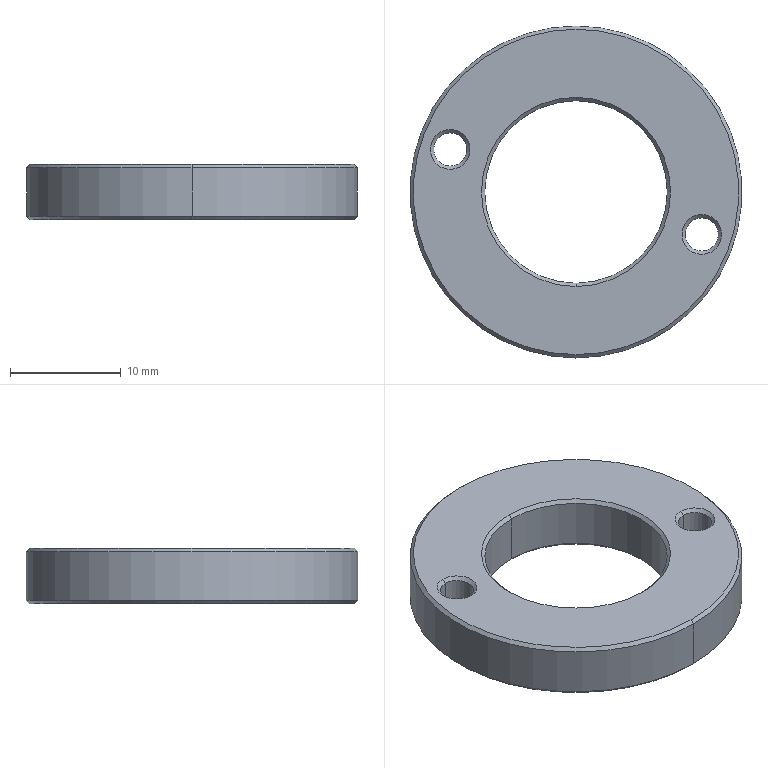Part | SolidWorks | features BaseBody 1 | 1 solid | 22 faces | box 30 x 30 x 5 mm | volume 2380 mm3 | cone 12 | cylinder 8 | plane 2 | commonest cylinder face diameters 3 x4 16.5 x2 30 x2
STEP:
#1=CARTESIAN_POINT('',(700.535,23.972,-71.23));
#2=VERTEX_POINT('',#1);
#3=CARTESIAN_POINT('',(700.535,53.372,-71.23));
#4=VERTEX_POINT('',#3);
#5=CARTESIAN_POINT('',(700.535,38.672,-71.23));
#6=DIRECTION('',(0.000000001,-0.000000003,1.));
#7=DIRECTION('',(0.,-1.,-0.000000003));
#8=AXIS2_PLACEMENT_3D('',#5,#6,#7);
#9=CIRCLE('',#8,14.7);
#10=EDGE_CURVE('',#2,#4,#9,.T.);
#11=ORIENTED_EDGE('',*,*,#10,.T.);
#12=CARTESIAN_POINT('',(700.535,53.672,-70.93));
#13=VERTEX_POINT('',#12);
#14=CARTESIAN_POINT('',(700.535,53.672,-70.93));
#15=DIRECTION('',(0.000000001,0.7071,0.7071));
#16=VECTOR('',#15,1000.);
#17=LINE('',#14,#16);
#18=EDGE_CURVE('',#4,#13,#17,.T.);
#19=ORIENTED_EDGE('',*,*,#18,.T.);
#20=CARTESIAN_POINT('',(700.535,23.672,-70.93));
#21=VERTEX_POINT('',#20);
#22=CARTESIAN_POINT('',(700.535,38.672,-70.93));
#23=DIRECTION('',(-0.000000001,0.000000003,-1.));
#24=DIRECTION('',(0.004352,-1.,-0.000000003));
#25=AXIS2_PLACEMENT_3D('',#22,#23,#24);
#26=CIRCLE('',#25,15.);
#27=EDGE_CURVE('',#13,#21,#26,.T.);
#28=ORIENTED_EDGE('',*,*,#27,.T.);
#29=CARTESIAN_POINT('',(700.535,23.672,-70.93));
#30=DIRECTION('',(0.000000001,-0.7071,0.7071));
#31=VECTOR('',#30,1000.);
#32=LINE('',#29,#31);
#33=EDGE_CURVE('',#2,#21,#32,.T.);
#34=ORIENTED_EDGE('',*,*,#33,.F.);
#35=EDGE_LOOP('',(#11,#19,#28,#34));
#36=FACE_OUTER_BOUND('',#35,.T.);
#37=CARTESIAN_POINT('',(700.535,38.672,-70.93));
#38=DIRECTION('',(0.000000001,-0.000000003,1.));
#39=DIRECTION('',(0.,-1.,-0.000000003));
#40=AXIS2_PLACEMENT_3D('',#37,#38,#39);
#41=CONICAL_SURFACE('',#40,15.,0.7854);
#42=ADVANCED_FACE('',(#36),#41,.T.);
#43=CARTESIAN_POINT('',(711.903,33.329,-71.23));
#44=VERTEX_POINT('',#43);
#45=CARTESIAN_POINT('',(711.903,36.329,-71.23));
#46=VERTEX_POINT('',#45);
#47=CARTESIAN_POINT('',(711.903,34.829,-71.23));
#48=DIRECTION('',(-0.000000001,0.000000003,-1.));
#49=DIRECTION('',(0.,-1.,-0.000000003));
#50=AXIS2_PLACEMENT_3D('',#47,#48,#49);
#51=CIRCLE('',#50,1.5);
#52=EDGE_CURVE('',#44,#46,#51,.T.);
#53=ORIENTED_EDGE('',*,*,#52,.T.);
#54=CARTESIAN_POINT('',(711.903,36.329,-66.53));
#55=VERTEX_POINT('',#54);
#56=CARTESIAN_POINT('',(711.903,36.329,-66.23));
#57=DIRECTION('',(0.000000001,-0.000000003,1.));
#58=VECTOR('',#57,1000.);
#59=LINE('',#56,#58);
#60=EDGE_CURVE('',#46,#55,#59,.T.);
#61=ORIENTED_EDGE('',*,*,#60,.T.);
#62=CARTESIAN_POINT('',(711.903,33.329,-66.53));
#63=VERTEX_POINT('',#62);
#64=CARTESIAN_POINT('',(711.903,34.829,-66.53));
#65=DIRECTION('',(-0.000000001,0.000000003,-1.));
#66=DIRECTION('',(0.,-1.,-0.000000003));
#67=AXIS2_PLACEMENT_3D('',#64,#65,#66);
#68=CIRCLE('',#67,1.5);
#69=EDGE_CURVE('',#63,#55,#68,.T.);
#70=ORIENTED_EDGE('',*,*,#69,.F.);
#71=CARTESIAN_POINT('',(711.903,33.329,-66.23));
#72=DIRECTION('',(0.000000001,-0.000000003,1.));
#73=VECTOR('',#72,1000.);
#74=LINE('',#71,#73);
#75=EDGE_CURVE('',#44,#63,#74,.T.);
#76=ORIENTED_EDGE('',*,*,#75,.F.);
#77=EDGE_LOOP('',(#53,#61,#70,#76));
#78=FACE_OUTER_BOUND('',#77,.T.);
#79=CARTESIAN_POINT('',(711.903,34.829,-66.23));
#80=DIRECTION('',(0.000000001,-0.000000003,1.));
#81=DIRECTION('',(0.,-1.,-0.000000003));
#82=AXIS2_PLACEMENT_3D('',#79,#80,#81);
#83=CYLINDRICAL_SURFACE('',#82,1.5);
#84=ADVANCED_FACE('',(#78),#83,.F.);
#85=CARTESIAN_POINT('',(689.167,41.015,-71.23));
#86=VERTEX_POINT('',#85);
#87=CARTESIAN_POINT('',(689.167,44.015,-71.23));
#88=VERTEX_POINT('',#87);
#89=CARTESIAN_POINT('',(689.167,42.515,-71.23));
#90=DIRECTION('',(-0.000000001,0.000000003,-1.));
#91=DIRECTION('',(0.,-1.,-0.000000003));
#92=AXIS2_PLACEMENT_3D('',#89,#90,#91);
#93=CIRCLE('',#92,1.5);
#94=EDGE_CURVE('',#86,#88,#93,.T.);
#95=ORIENTED_EDGE('',*,*,#94,.T.);
#96=CARTESIAN_POINT('',(689.167,44.015,-66.53));
#97=VERTEX_POINT('',#96);
#98=CARTESIAN_POINT('',(689.167,44.015,-66.23));
#99=DIRECTION('',(0.000000001,-0.000000003,1.));
#100=VECTOR('',#99,1000.);
#101=LINE('',#98,#100);
#102=EDGE_CURVE('',#88,#97,#101,.T.);
#103=ORIENTED_EDGE('',*,*,#102,.T.);
#104=CARTESIAN_POINT('',(689.167,41.015,-66.53));
#105=VERTEX_POINT('',#104);
#106=CARTESIAN_POINT('',(689.167,42.515,-66.53));
#107=DIRECTION('',(-0.000000001,0.000000003,-1.));
#108=DIRECTION('',(0.,-1.,-0.000000003));
#109=AXIS2_PLACEMENT_3D('',#106,#107,#108);
#110=CIRCLE('',#109,1.5);
#111=EDGE_CURVE('',#105,#97,#110,.T.);
#112=ORIENTED_EDGE('',*,*,#111,.F.);
#113=CARTESIAN_POINT('',(689.167,41.015,-66.23));
#114=DIRECTION('',(0.000000001,-0.000000003,1.));
#115=VECTOR('',#114,1000.);
#116=LINE('',#113,#115);
#117=EDGE_CURVE('',#86,#105,#116,.T.);
#118=ORIENTED_EDGE('',*,*,#117,.F.);
#119=EDGE_LOOP('',(#95,#103,#112,#118));
#120=FACE_OUTER_BOUND('',#119,.T.);
#121=CARTESIAN_POINT('',(689.167,42.515,-66.23));
#122=DIRECTION('',(0.000000001,-0.000000003,1.));
#123=DIRECTION('',(0.,-1.,-0.000000003));
#124=AXIS2_PLACEMENT_3D('',#121,#122,#123);
#125=CYLINDRICAL_SURFACE('',#124,1.5);
#126=ADVANCED_FACE('',(#120),#125,.F.);
#127=CARTESIAN_POINT('',(700.535,30.422,-70.93));
#128=VERTEX_POINT('',#127);
#129=CARTESIAN_POINT('',(700.535,46.922,-70.93));
#130=VERTEX_POINT('',#129);
#131=CARTESIAN_POINT('',(700.535,38.672,-70.93));
#132=DIRECTION('',(-0.000000001,0.000000003,-1.));
#133=DIRECTION('',(-0.004352,1.,0.000000003));
#134=AXIS2_PLACEMENT_3D('',#131,#132,#133);
#135=CIRCLE('',#134,8.25);
#136=EDGE_CURVE('',#128,#130,#135,.T.);
#137=ORIENTED_EDGE('',*,*,#136,.F.);
#138=CARTESIAN_POINT('',(700.535,30.122,-71.23));
#139=VERTEX_POINT('',#138);
#140=CARTESIAN_POINT('',(700.535,30.122,-71.23));
#141=DIRECTION('',(-0.000000001,-0.7071,-0.7071));
#142=VECTOR('',#141,1000.);
#143=LINE('',#140,#142);
#144=EDGE_CURVE('',#128,#139,#143,.T.);
#145=ORIENTED_EDGE('',*,*,#144,.T.);
#146=CARTESIAN_POINT('',(700.535,47.222,-71.23));
#147=VERTEX_POINT('',#146);
#148=CARTESIAN_POINT('',(700.535,38.672,-71.23));
#149=DIRECTION('',(-0.000000001,0.000000003,-1.));
#150=DIRECTION('',(0.,1.,0.000000003));
#151=AXIS2_PLACEMENT_3D('',#148,#149,#150);
#152=CIRCLE('',#151,8.55);
#153=EDGE_CURVE('',#139,#147,#152,.T.);
#154=ORIENTED_EDGE('',*,*,#153,.T.);
#155=CARTESIAN_POINT('',(700.535,47.222,-71.23));
#156=DIRECTION('',(-0.000000001,0.7071,-0.7071));
#157=VECTOR('',#156,1000.);
#158=LINE('',#155,#157);
#159=EDGE_CURVE('',#130,#147,#158,.T.);
#160=ORIENTED_EDGE('',*,*,#159,.F.);
#161=EDGE_LOOP('',(#137,#145,#154,#160));
#162=FACE_OUTER_BOUND('',#161,.T.);
#163=CARTESIAN_POINT('',(700.535,38.672,-71.23));
#164=DIRECTION('',(-0.000000001,0.000000003,-1.));
#165=DIRECTION('',(0.,1.,0.000000003));
#166=AXIS2_PLACEMENT_3D('',#163,#164,#165);
#167=CONICAL_SURFACE('',#166,8.55,0.7854);
#168=ADVANCED_FACE('',(#162),#167,.F.);
#169=CARTESIAN_POINT('',(700.535,53.672,-66.53));
#170=VERTEX_POINT('',#169);
#171=CARTESIAN_POINT('',(700.535,23.672,-66.53));
#172=VERTEX_POINT('',#171);
#173=CARTESIAN_POINT('',(700.535,38.672,-66.53));
#174=DIRECTION('',(-0.000000001,0.000000003,-1.));
#175=DIRECTION('',(0.,1.,0.000000003));
#176=AXIS2_PLACEMENT_3D('',#173,#174,#175);
#177=CIRCLE('',#176,15.);
#178=EDGE_CURVE('',#170,#172,#177,.T.);
#179=ORIENTED_EDGE('',*,*,#178,.T.);
#180=CARTESIAN_POINT('',(700.535,23.672,-71.23));
#181=DIRECTION('',(-0.000000001,0.000000003,-1.));
#182=VECTOR('',#181,1000.);
#183=LINE('',#180,#182);
#184=EDGE_CURVE('',#172,#21,#183,.T.);
#185=ORIENTED_EDGE('',*,*,#184,.T.);
#186=ORIENTED_EDGE('',*,*,#27,.F.);
#187=CARTESIAN_POINT('',(700.535,53.672,-71.23));
#188=DIRECTION('',(-0.000000001,0.000000003,-1.));
#189=VECTOR('',#188,1000.);
#190=LINE('',#187,#189);
#191=EDGE_CURVE('',#170,#13,#190,.T.);
#192=ORIENTED_EDGE('',*,*,#191,.F.);
#193=EDGE_LOOP('',(#179,#185,#186,#192));
#194=FACE_OUTER_BOUND('',#193,.T.);
#195=CARTESIAN_POINT('',(700.535,38.672,-71.23));
#196=DIRECTION('',(-0.000000001,0.000000003,-1.));
#197=DIRECTION('',(0.,1.,0.000000003));
#198=AXIS2_PLACEMENT_3D('',#195,#196,#197);
#199=CYLINDRICAL_SURFACE('',#198,15.);
#200=ADVANCED_FACE('',(#194),#199,.T.);
#201=ORIENTED_EDGE('',*,*,#69,.T.);
#202=CARTESIAN_POINT('',(711.903,36.629,-66.23));
#203=VERTEX_POINT('',#202);
#204=CARTESIAN_POINT('',(711.903,36.629,-66.23));
#205=DIRECTION('',(0.000000001,0.7071,0.7071));
#206=VECTOR('',#205,1000.);
#207=LINE('',#204,#206);
#208=EDGE_CURVE('',#55,#203,#207,.T.);
#209=ORIENTED_EDGE('',*,*,#208,.T.);
#210=CARTESIAN_POINT('',(711.903,33.029,-66.23));
#211=VERTEX_POINT('',#210);
#212=CARTESIAN_POINT('',(711.903,34.829,-66.23));
#213=DIRECTION('',(-0.000000001,0.000000003,-1.));
#214=DIRECTION('',(0.,-1.,-0.000000003));
#215=AXIS2_PLACEMENT_3D('',#212,#213,#214);
#216=CIRCLE('',#215,1.8);
#217=EDGE_CURVE('',#211,#203,#216,.T.);
#218=ORIENTED_EDGE('',*,*,#217,.F.);
#219=CARTESIAN_POINT('',(711.903,33.029,-66.23));
#220=DIRECTION('',(0.000000001,-0.7071,0.7071));
#221=VECTOR('',#220,1000.);
#222=LINE('',#219,#221);
#223=EDGE_CURVE('',#63,#211,#222,.T.);
#224=ORIENTED_EDGE('',*,*,#223,.F.);
#225=EDGE_LOOP('',(#201,#209,#218,#224));
#226=FACE_OUTER_BOUND('',#225,.T.);
#227=CARTESIAN_POINT('',(711.903,34.829,-66.23));
#228=DIRECTION('',(0.000000001,-0.000000003,1.));
#229=DIRECTION('',(0.,-1.,-0.000000003));
#230=AXIS2_PLACEMENT_3D('',#227,#228,#229);
#231=CONICAL_SURFACE('',#230,1.8,0.7854);
#232=ADVANCED_FACE('',(#226),#231,.F.);
#233=ORIENTED_EDGE('',*,*,#111,.T.);
#234=CARTESIAN_POINT('',(689.167,44.315,-66.23));
#235=VERTEX_POINT('',#234);
#236=CARTESIAN_POINT('',(689.167,44.315,-66.23));
#237=DIRECTION('',(0.000000001,0.7071,0.7071));
#238=VECTOR('',#237,1000.);
#239=LINE('',#236,#238);
#240=EDGE_CURVE('',#97,#235,#239,.T.);
#241=ORIENTED_EDGE('',*,*,#240,.T.);
#242=CARTESIAN_POINT('',(689.167,40.715,-66.23));
#243=VERTEX_POINT('',#242);
#244=CARTESIAN_POINT('',(689.167,42.515,-66.23));
#245=DIRECTION('',(-0.000000001,0.000000003,-1.));
#246=DIRECTION('',(0.,-1.,-0.000000003));
#247=AXIS2_PLACEMENT_3D('',#244,#245,#246);
#248=CIRCLE('',#247,1.8);
#249=EDGE_CURVE('',#243,#235,#248,.T.);
#250=ORIENTED_EDGE('',*,*,#249,.F.);
#251=CARTESIAN_POINT('',(689.167,40.715,-66.23));
#252=DIRECTION('',(0.000000001,-0.7071,0.7071));
#253=VECTOR('',#252,1000.);
#254=LINE('',#251,#253);
#255=EDGE_CURVE('',#105,#243,#254,.T.);
#256=ORIENTED_EDGE('',*,*,#255,.F.);
#257=EDGE_LOOP('',(#233,#241,#250,#256));
#258=FACE_OUTER_BOUND('',#257,.T.);
#259=CARTESIAN_POINT('',(689.167,42.515,-66.23));
#260=DIRECTION('',(0.000000001,-0.000000003,1.));
#261=DIRECTION('',(0.,-1.,-0.000000003));
#262=AXIS2_PLACEMENT_3D('',#259,#260,#261);
#263=CONICAL_SURFACE('',#262,1.8,0.7854);
#264=ADVANCED_FACE('',(#258),#263,.F.);
#265=CARTESIAN_POINT('',(700.535,30.422,-66.53));
#266=VERTEX_POINT('',#265);
#267=CARTESIAN_POINT('',(700.535,46.922,-66.53));
#268=VERTEX_POINT('',#267);
#269=CARTESIAN_POINT('',(700.535,38.672,-66.53));
#270=DIRECTION('',(-0.000000001,0.000000003,-1.));
#271=DIRECTION('',(0.,1.,0.000000003));
#272=AXIS2_PLACEMENT_3D('',#269,#270,#271);
#273=CIRCLE('',#272,8.25);
#274=EDGE_CURVE('',#266,#268,#273,.T.);
#275=ORIENTED_EDGE('',*,*,#274,.F.);
#276=CARTESIAN_POINT('',(700.535,30.422,-68.73));
#277=DIRECTION('',(-0.000000001,0.000000003,-1.));
#278=VECTOR('',#277,1000.);
#279=LINE('',#276,#278);
#280=EDGE_CURVE('',#266,#128,#279,.T.);
#281=ORIENTED_EDGE('',*,*,#280,.T.);
#282=ORIENTED_EDGE('',*,*,#136,.T.);
#283=CARTESIAN_POINT('',(700.535,46.922,-68.73));
#284=DIRECTION('',(-0.000000001,0.000000003,-1.));
#285=VECTOR('',#284,1000.);
#286=LINE('',#283,#285);
#287=EDGE_CURVE('',#268,#130,#286,.T.);
#288=ORIENTED_EDGE('',*,*,#287,.F.);
#289=EDGE_LOOP('',(#275,#281,#282,#288));
#290=FACE_OUTER_BOUND('',#289,.T.);
#291=CARTESIAN_POINT('',(700.535,38.672,-68.73));
#292=DIRECTION('',(-0.000000001,0.000000003,-1.));
#293=DIRECTION('',(0.,1.,0.000000003));
#294=AXIS2_PLACEMENT_3D('',#291,#292,#293);
#295=CYLINDRICAL_SURFACE('',#294,8.25);
#296=ADVANCED_FACE('',(#290),#295,.F.);
#297=CARTESIAN_POINT('',(700.535,53.372,-66.23));
#298=VERTEX_POINT('',#297);
#299=CARTESIAN_POINT('',(700.535,23.972,-66.23));
#300=VERTEX_POINT('',#299);
#301=CARTESIAN_POINT('',(700.535,38.672,-66.23));
#302=DIRECTION('',(-0.000000001,0.000000003,-1.));
#303=DIRECTION('',(0.,1.,0.000000003));
#304=AXIS2_PLACEMENT_3D('',#301,#302,#303);
#305=CIRCLE('',#304,14.7);
#306=EDGE_CURVE('',#298,#300,#305,.T.);
#307=ORIENTED_EDGE('',*,*,#306,.T.);
#308=CARTESIAN_POINT('',(700.535,23.672,-66.53));
#309=DIRECTION('',(-0.000000001,-0.7071,-0.7071));
#310=VECTOR('',#309,1000.);
#311=LINE('',#308,#310);
#312=EDGE_CURVE('',#300,#172,#311,.T.);
#313=ORIENTED_EDGE('',*,*,#312,.T.);
#314=ORIENTED_EDGE('',*,*,#178,.F.);
#315=CARTESIAN_POINT('',(700.535,53.672,-66.53));
#316=DIRECTION('',(-0.000000001,0.7071,-0.7071));
#317=VECTOR('',#316,1000.);
#318=LINE('',#315,#317);
#319=EDGE_CURVE('',#298,#170,#318,.T.);
#320=ORIENTED_EDGE('',*,*,#319,.F.);
#321=EDGE_LOOP('',(#307,#313,#314,#320));
#322=FACE_OUTER_BOUND('',#321,.T.);
#323=CARTESIAN_POINT('',(700.535,38.672,-66.53));
#324=DIRECTION('',(-0.000000001,0.000000003,-1.));
#325=DIRECTION('',(0.,1.,0.000000003));
#326=AXIS2_PLACEMENT_3D('',#323,#324,#325);
#327=CONICAL_SURFACE('',#326,15.,0.7854);
#328=ADVANCED_FACE('',(#322),#327,.T.);
#329=ORIENTED_EDGE('',*,*,#274,.T.);
#330=CARTESIAN_POINT('',(700.535,47.222,-66.23));
#331=VERTEX_POINT('',#330);
#332=CARTESIAN_POINT('',(700.535,47.222,-66.23));
#333=DIRECTION('',(0.000000001,0.7071,0.7071));
#334=VECTOR('',#333,1000.);
#335=LINE('',#332,#334);
#336=EDGE_CURVE('',#268,#331,#335,.T.);
#337=ORIENTED_EDGE('',*,*,#336,.T.);
#338=CARTESIAN_POINT('',(700.535,30.122,-66.23));
#339=VERTEX_POINT('',#338);
#340=CARTESIAN_POINT('',(700.535,38.672,-66.23));
#341=DIRECTION('',(-0.000000001,0.000000003,-1.));
#342=DIRECTION('',(0.,-1.,-0.000000003));
#343=AXIS2_PLACEMENT_3D('',#340,#341,#342);
#344=CIRCLE('',#343,8.55);
#345=EDGE_CURVE('',#339,#331,#344,.T.);
#346=ORIENTED_EDGE('',*,*,#345,.F.);
#347=CARTESIAN_POINT('',(700.535,30.122,-66.23));
#348=DIRECTION('',(0.000000001,-0.7071,0.7071));
#349=VECTOR('',#348,1000.);
#350=LINE('',#347,#349);
#351=EDGE_CURVE('',#266,#339,#350,.T.);
#352=ORIENTED_EDGE('',*,*,#351,.F.);
#353=EDGE_LOOP('',(#329,#337,#346,#352));
#354=FACE_OUTER_BOUND('',#353,.T.);
#355=CARTESIAN_POINT('',(700.535,38.672,-66.23));
#356=DIRECTION('',(0.000000001,-0.000000003,1.));
#357=DIRECTION('',(0.,-1.,-0.000000003));
#358=AXIS2_PLACEMENT_3D('',#355,#356,#357);
#359=CONICAL_SURFACE('',#358,8.55,0.7854);
#360=ADVANCED_FACE('',(#354),#359,.F.);
#361=ORIENTED_EDGE('',*,*,#10,.F.);
#362=CARTESIAN_POINT('',(700.535,38.672,-71.23));
#363=DIRECTION('',(0.000000001,-0.000000003,1.));
#364=DIRECTION('',(0.,-1.,-0.000000003));
#365=AXIS2_PLACEMENT_3D('',#362,#363,#364);
#366=CIRCLE('',#365,14.7);
#367=EDGE_CURVE('',#4,#2,#366,.T.);
#368=ORIENTED_EDGE('',*,*,#367,.F.);
#369=EDGE_LOOP('',(#361,#368));
#370=FACE_OUTER_BOUND('',#369,.T.);
#371=ORIENTED_EDGE('',*,*,#52,.F.);
#372=CARTESIAN_POINT('',(711.903,34.829,-71.23));
#373=DIRECTION('',(-0.000000001,0.000000003,-1.));
#374=DIRECTION('',(0.,-1.,-0.000000003));
#375=AXIS2_PLACEMENT_3D('',#372,#373,#374);
#376=CIRCLE('',#375,1.5);
#377=EDGE_CURVE('',#46,#44,#376,.T.);
#378=ORIENTED_EDGE('',*,*,#377,.F.);
#379=EDGE_LOOP('',(#371,#378));
#380=FACE_BOUND('',#379,.T.);
#381=ORIENTED_EDGE('',*,*,#94,.F.);
#382=CARTESIAN_POINT('',(689.167,42.515,-71.23));
#383=DIRECTION('',(-0.000000001,0.000000003,-1.));
#384=DIRECTION('',(0.,-1.,-0.000000003));
#385=AXIS2_PLACEMENT_3D('',#382,#383,#384);
#386=CIRCLE('',#385,1.5);
#387=EDGE_CURVE('',#88,#86,#386,.T.);
#388=ORIENTED_EDGE('',*,*,#387,.F.);
#389=EDGE_LOOP('',(#381,#388));
#390=FACE_BOUND('',#389,.T.);
#391=CARTESIAN_POINT('',(700.535,38.672,-71.23));
#392=DIRECTION('',(-0.000000001,0.000000003,-1.));
#393=DIRECTION('',(0.,1.,0.000000003));
#394=AXIS2_PLACEMENT_3D('',#391,#392,#393);
#395=CIRCLE('',#394,8.55);
#396=EDGE_CURVE('',#147,#139,#395,.T.);
#397=ORIENTED_EDGE('',*,*,#396,.F.);
#398=ORIENTED_EDGE('',*,*,#153,.F.);
#399=EDGE_LOOP('',(#397,#398));
#400=FACE_BOUND('',#399,.T.);
#401=CARTESIAN_POINT('',(700.535,38.672,-71.23));
#402=DIRECTION('',(0.000000001,-0.000000003,1.));
#403=DIRECTION('',(0.,-1.,-0.000000003));
#404=AXIS2_PLACEMENT_3D('',#401,#402,#403);
#405=PLANE('',#404);
#406=ADVANCED_FACE('',(#370,#380,#390,#400),#405,.F.);
#407=ORIENTED_EDGE('',*,*,#18,.F.);
#408=ORIENTED_EDGE('',*,*,#367,.T.);
#409=ORIENTED_EDGE('',*,*,#33,.T.);
#410=CARTESIAN_POINT('',(700.535,38.672,-70.93));
#411=DIRECTION('',(-0.000000001,0.000000003,-1.));
#412=DIRECTION('',(0.004352,-1.,-0.000000003));
#413=AXIS2_PLACEMENT_3D('',#410,#411,#412);
#414=CIRCLE('',#413,15.);
#415=EDGE_CURVE('',#21,#13,#414,.T.);
#416=ORIENTED_EDGE('',*,*,#415,.T.);
#417=EDGE_LOOP('',(#407,#408,#409,#416));
#418=FACE_OUTER_BOUND('',#417,.T.);
#419=CARTESIAN_POINT('',(700.535,38.672,-70.93));
#420=DIRECTION('',(0.000000001,-0.000000003,1.));
#421=DIRECTION('',(0.,-1.,-0.000000003));
#422=AXIS2_PLACEMENT_3D('',#419,#420,#421);
#423=CONICAL_SURFACE('',#422,15.,0.7854);
#424=ADVANCED_FACE('',(#418),#423,.T.);
#425=ORIENTED_EDGE('',*,*,#60,.F.);
#426=ORIENTED_EDGE('',*,*,#377,.T.);
#427=ORIENTED_EDGE('',*,*,#75,.T.);
#428=CARTESIAN_POINT('',(711.903,34.829,-66.53));
#429=DIRECTION('',(-0.000000001,0.000000003,-1.));
#430=DIRECTION('',(0.,-1.,-0.000000003));
#431=AXIS2_PLACEMENT_3D('',#428,#429,#430);
#432=CIRCLE('',#431,1.5);
#433=EDGE_CURVE('',#55,#63,#432,.T.);
#434=ORIENTED_EDGE('',*,*,#433,.F.);
#435=EDGE_LOOP('',(#425,#426,#427,#434));
#436=FACE_OUTER_BOUND('',#435,.T.);
#437=CARTESIAN_POINT('',(711.903,34.829,-66.23));
#438=DIRECTION('',(0.000000001,-0.000000003,1.));
#439=DIRECTION('',(0.,-1.,-0.000000003));
#440=AXIS2_PLACEMENT_3D('',#437,#438,#439);
#441=CYLINDRICAL_SURFACE('',#440,1.5);
#442=ADVANCED_FACE('',(#436),#441,.F.);
#443=ORIENTED_EDGE('',*,*,#102,.F.);
#444=ORIENTED_EDGE('',*,*,#387,.T.);
#445=ORIENTED_EDGE('',*,*,#117,.T.);
#446=CARTESIAN_POINT('',(689.167,42.515,-66.53));
#447=DIRECTION('',(-0.000000001,0.000000003,-1.));
#448=DIRECTION('',(0.,-1.,-0.000000003));
#449=AXIS2_PLACEMENT_3D('',#446,#447,#448);
#450=CIRCLE('',#449,1.5);
#451=EDGE_CURVE('',#97,#105,#450,.T.);
#452=ORIENTED_EDGE('',*,*,#451,.F.);
#453=EDGE_LOOP('',(#443,#444,#445,#452));
#454=FACE_OUTER_BOUND('',#453,.T.);
#455=CARTESIAN_POINT('',(689.167,42.515,-66.23));
#456=DIRECTION('',(0.000000001,-0.000000003,1.));
#457=DIRECTION('',(0.,-1.,-0.000000003));
#458=AXIS2_PLACEMENT_3D('',#455,#456,#457);
#459=CYLINDRICAL_SURFACE('',#458,1.5);
#460=ADVANCED_FACE('',(#454),#459,.F.);
#461=ORIENTED_EDGE('',*,*,#144,.F.);
#462=CARTESIAN_POINT('',(700.535,38.672,-70.93));
#463=DIRECTION('',(-0.000000001,0.000000003,-1.));
#464=DIRECTION('',(-0.004352,1.,0.000000003));
#465=AXIS2_PLACEMENT_3D('',#462,#463,#464);
#466=CIRCLE('',#465,8.25);
#467=EDGE_CURVE('',#130,#128,#466,.T.);
#468=ORIENTED_EDGE('',*,*,#467,.F.);
#469=ORIENTED_EDGE('',*,*,#159,.T.);
#470=ORIENTED_EDGE('',*,*,#396,.T.);
#471=EDGE_LOOP('',(#461,#468,#469,#470));
#472=FACE_OUTER_BOUND('',#471,.T.);
#473=CARTESIAN_POINT('',(700.535,38.672,-71.23));
#474=DIRECTION('',(-0.000000001,0.000000003,-1.));
#475=DIRECTION('',(0.,1.,0.000000003));
#476=AXIS2_PLACEMENT_3D('',#473,#474,#475);
#477=CONICAL_SURFACE('',#476,8.55,0.7854);
#478=ADVANCED_FACE('',(#472),#477,.F.);
#479=ORIENTED_EDGE('',*,*,#184,.F.);
#480=CARTESIAN_POINT('',(700.535,38.672,-66.53));
#481=DIRECTION('',(-0.000000001,0.000000003,-1.));
#482=DIRECTION('',(0.,1.,0.000000003));
#483=AXIS2_PLACEMENT_3D('',#480,#481,#482);
#484=CIRCLE('',#483,15.);
#485=EDGE_CURVE('',#172,#170,#484,.T.);
#486=ORIENTED_EDGE('',*,*,#485,.T.);
#487=ORIENTED_EDGE('',*,*,#191,.T.);
#488=ORIENTED_EDGE('',*,*,#415,.F.);
#489=EDGE_LOOP('',(#479,#486,#487,#488));
#490=FACE_OUTER_BOUND('',#489,.T.);
#491=CARTESIAN_POINT('',(700.535,38.672,-71.23));
#492=DIRECTION('',(-0.000000001,0.000000003,-1.));
#493=DIRECTION('',(0.,1.,0.000000003));
#494=AXIS2_PLACEMENT_3D('',#491,#492,#493);
#495=CYLINDRICAL_SURFACE('',#494,15.);
#496=ADVANCED_FACE('',(#490),#495,.T.);
#497=ORIENTED_EDGE('',*,*,#208,.F.);
#498=ORIENTED_EDGE('',*,*,#433,.T.);
#499=ORIENTED_EDGE('',*,*,#223,.T.);
#500=CARTESIAN_POINT('',(711.903,34.829,-66.23));
#501=DIRECTION('',(-0.000000001,0.000000003,-1.));
#502=DIRECTION('',(0.,-1.,-0.000000003));
#503=AXIS2_PLACEMENT_3D('',#500,#501,#502);
#504=CIRCLE('',#503,1.8);
#505=EDGE_CURVE('',#203,#211,#504,.T.);
#506=ORIENTED_EDGE('',*,*,#505,.F.);
#507=EDGE_LOOP('',(#497,#498,#499,#506));
#508=FACE_OUTER_BOUND('',#507,.T.);
#509=CARTESIAN_POINT('',(711.903,34.829,-66.23));
#510=DIRECTION('',(0.000000001,-0.000000003,1.));
#511=DIRECTION('',(0.,-1.,-0.000000003));
#512=AXIS2_PLACEMENT_3D('',#509,#510,#511);
#513=CONICAL_SURFACE('',#512,1.8,0.7854);
#514=ADVANCED_FACE('',(#508),#513,.F.);
#515=ORIENTED_EDGE('',*,*,#240,.F.);
#516=ORIENTED_EDGE('',*,*,#451,.T.);
#517=ORIENTED_EDGE('',*,*,#255,.T.);
#518=CARTESIAN_POINT('',(689.167,42.515,-66.23));
#519=DIRECTION('',(-0.000000001,0.000000003,-1.));
#520=DIRECTION('',(0.,-1.,-0.000000003));
#521=AXIS2_PLACEMENT_3D('',#518,#519,#520);
#522=CIRCLE('',#521,1.8);
#523=EDGE_CURVE('',#235,#243,#522,.T.);
#524=ORIENTED_EDGE('',*,*,#523,.F.);
#525=EDGE_LOOP('',(#515,#516,#517,#524));
#526=FACE_OUTER_BOUND('',#525,.T.);
#527=CARTESIAN_POINT('',(689.167,42.515,-66.23));
#528=DIRECTION('',(0.000000001,-0.000000003,1.));
#529=DIRECTION('',(0.,-1.,-0.000000003));
#530=AXIS2_PLACEMENT_3D('',#527,#528,#529);
#531=CONICAL_SURFACE('',#530,1.8,0.7854);
#532=ADVANCED_FACE('',(#526),#531,.F.);
#533=ORIENTED_EDGE('',*,*,#280,.F.);
#534=CARTESIAN_POINT('',(700.535,38.672,-66.53));
#535=DIRECTION('',(-0.000000001,0.000000003,-1.));
#536=DIRECTION('',(0.,1.,0.000000003));
#537=AXIS2_PLACEMENT_3D('',#534,#535,#536);
#538=CIRCLE('',#537,8.25);
#539=EDGE_CURVE('',#268,#266,#538,.T.);
#540=ORIENTED_EDGE('',*,*,#539,.F.);
#541=ORIENTED_EDGE('',*,*,#287,.T.);
#542=ORIENTED_EDGE('',*,*,#467,.T.);
#543=EDGE_LOOP('',(#533,#540,#541,#542));
#544=FACE_OUTER_BOUND('',#543,.T.);
#545=CARTESIAN_POINT('',(700.535,38.672,-68.73));
#546=DIRECTION('',(-0.000000001,0.000000003,-1.));
#547=DIRECTION('',(0.,1.,0.000000003));
#548=AXIS2_PLACEMENT_3D('',#545,#546,#547);
#549=CYLINDRICAL_SURFACE('',#548,8.25);
#550=ADVANCED_FACE('',(#544),#549,.F.);
#551=ORIENTED_EDGE('',*,*,#312,.F.);
#552=CARTESIAN_POINT('',(700.535,38.672,-66.23));
#553=DIRECTION('',(-0.000000001,0.000000003,-1.));
#554=DIRECTION('',(0.,1.,0.000000003));
#555=AXIS2_PLACEMENT_3D('',#552,#553,#554);
#556=CIRCLE('',#555,14.7);
#557=EDGE_CURVE('',#300,#298,#556,.T.);
#558=ORIENTED_EDGE('',*,*,#557,.T.);
#559=ORIENTED_EDGE('',*,*,#319,.T.);
#560=ORIENTED_EDGE('',*,*,#485,.F.);
#561=EDGE_LOOP('',(#551,#558,#559,#560));
#562=FACE_OUTER_BOUND('',#561,.T.);
#563=CARTESIAN_POINT('',(700.535,38.672,-66.53));
#564=DIRECTION('',(-0.000000001,0.000000003,-1.));
#565=DIRECTION('',(0.,1.,0.000000003));
#566=AXIS2_PLACEMENT_3D('',#563,#564,#565);
#567=CONICAL_SURFACE('',#566,15.,0.7854);
#568=ADVANCED_FACE('',(#562),#567,.T.);
#569=ORIENTED_EDGE('',*,*,#217,.T.);
#570=ORIENTED_EDGE('',*,*,#505,.T.);
#571=EDGE_LOOP('',(#569,#570));
#572=FACE_BOUND('',#571,.T.);
#573=ORIENTED_EDGE('',*,*,#345,.T.);
#574=CARTESIAN_POINT('',(700.535,38.672,-66.23));
#575=DIRECTION('',(-0.000000001,0.000000003,-1.));
#576=DIRECTION('',(0.,-1.,-0.000000003));
#577=AXIS2_PLACEMENT_3D('',#574,#575,#576);
#578=CIRCLE('',#577,8.55);
#579=EDGE_CURVE('',#331,#339,#578,.T.);
#580=ORIENTED_EDGE('',*,*,#579,.T.);
#581=EDGE_LOOP('',(#573,#580));
#582=FACE_BOUND('',#581,.T.);
#583=ORIENTED_EDGE('',*,*,#306,.F.);
#584=ORIENTED_EDGE('',*,*,#557,.F.);
#585=EDGE_LOOP('',(#583,#584));
#586=FACE_OUTER_BOUND('',#585,.T.);
#587=ORIENTED_EDGE('',*,*,#249,.T.);
#588=ORIENTED_EDGE('',*,*,#523,.T.);
#589=EDGE_LOOP('',(#587,#588));
#590=FACE_BOUND('',#589,.T.);
#591=CARTESIAN_POINT('',(700.535,38.672,-66.23));
#592=DIRECTION('',(0.000000001,-0.000000003,1.));
#593=DIRECTION('',(0.,-1.,-0.000000003));
#594=AXIS2_PLACEMENT_3D('',#591,#592,#593);
#595=PLANE('',#594);
#596=ADVANCED_FACE('',(#572,#582,#586,#590),#595,.T.);
#597=ORIENTED_EDGE('',*,*,#336,.F.);
#598=ORIENTED_EDGE('',*,*,#539,.T.);
#599=ORIENTED_EDGE('',*,*,#351,.T.);
#600=ORIENTED_EDGE('',*,*,#579,.F.);
#601=EDGE_LOOP('',(#597,#598,#599,#600));
#602=FACE_OUTER_BOUND('',#601,.T.);
#603=CARTESIAN_POINT('',(700.535,38.672,-66.23));
#604=DIRECTION('',(0.000000001,-0.000000003,1.));
#605=DIRECTION('',(0.,-1.,-0.000000003));
#606=AXIS2_PLACEMENT_3D('',#603,#604,#605);
#607=CONICAL_SURFACE('',#606,8.55,0.7854);
#608=ADVANCED_FACE('',(#602),#607,.F.);
#609=CLOSED_SHELL('',(#42,#84,#126,#168,#200,#232,#264,#296,#328,#360,#406,#424,#442,#460,#478,#496,#514,#532,#550,#568,#596,#608));
#610=MANIFOLD_SOLID_BREP('',#609);
#611=CARTESIAN_POINT('',(0.,0.,0.));
#612=DIRECTION('',(0.,0.,1.));
#613=DIRECTION('',(1.,0.,0.));
#614=AXIS2_PLACEMENT_3D('',#611,#612,#613);
#615=(LENGTH_UNIT()NAMED_UNIT(*)SI_UNIT(.MILLI.,.METRE.));
#616=UNCERTAINTY_MEASURE_WITH_UNIT(LENGTH_MEASURE(0.00001),#615,'','');
#617=(NAMED_UNIT(*)PLANE_ANGLE_UNIT()SI_UNIT($,.RADIAN.));
#618=(NAMED_UNIT(*)SI_UNIT($,.STERADIAN.)SOLID_ANGLE_UNIT());
#619=(GEOMETRIC_REPRESENTATION_CONTEXT(3)GLOBAL_UNCERTAINTY_ASSIGNED_CONTEXT((#616))GLOBAL_UNIT_ASSIGNED_CONTEXT((#615,#617,#618))REPRESENTATION_CONTEXT('',''));
#620=ADVANCED_BREP_SHAPE_REPRESENTATION('',(#610,#614),#619);